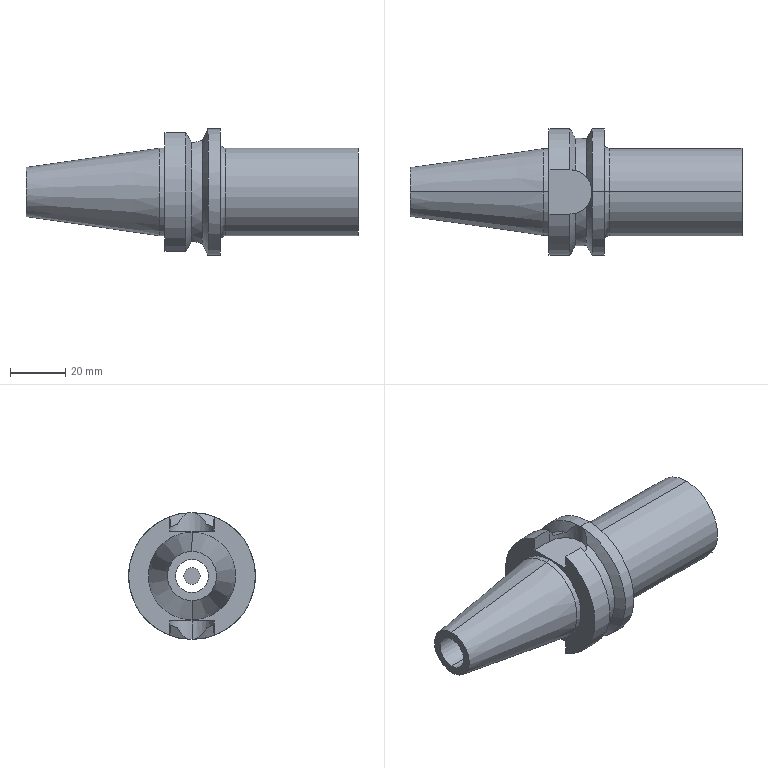Part | SolidWorks | features ICE 5, Fillet 1, MirrorPattern 1, RefAxis 1, Revolution 1 | 2 solids | 40 faces | box 120.4 x 46 x 46 mm | volume 69900 mm3 | cylinder 19 | plane 13 | cone 6 | torus 2 | commonest cylinder face diameters 46 x4 16.1 x3 6 x2 12 x2 24 x2 31.75 x2
STEP:
#1=CARTESIAN_POINT('',(90.4,0.,12.));
#2=VERTEX_POINT('',#1);
#3=CARTESIAN_POINT('',(90.4,0.,-12.));
#4=VERTEX_POINT('',#3);
#5=CARTESIAN_POINT('',(90.4,0.,0.));
#6=DIRECTION('',(1.,0.,0.));
#7=DIRECTION('',(0.,0.,-1.));
#8=AXIS2_PLACEMENT_3D('',#5,#6,#7);
#9=CIRCLE('',#8,12.);
#10=EDGE_CURVE('',#2,#4,#9,.T.);
#11=ORIENTED_EDGE('',*,*,#10,.F.);
#12=CARTESIAN_POINT('',(120.4,0.,12.));
#13=VERTEX_POINT('',#12);
#14=CARTESIAN_POINT('',(90.4,0.,12.));
#15=DIRECTION('',(1.,0.,0.));
#16=VECTOR('',#15,1000.);
#17=LINE('',#14,#16);
#18=EDGE_CURVE('',#2,#13,#17,.T.);
#19=ORIENTED_EDGE('',*,*,#18,.T.);
#20=CARTESIAN_POINT('',(120.4,0.,-12.));
#21=VERTEX_POINT('',#20);
#22=CARTESIAN_POINT('',(120.4,0.,0.));
#23=DIRECTION('',(1.,0.,0.));
#24=DIRECTION('',(0.,0.,-1.));
#25=AXIS2_PLACEMENT_3D('',#22,#23,#24);
#26=CIRCLE('',#25,12.);
#27=EDGE_CURVE('',#13,#21,#26,.T.);
#28=ORIENTED_EDGE('',*,*,#27,.T.);
#29=CARTESIAN_POINT('',(90.4,0.,-12.));
#30=DIRECTION('',(1.,0.,0.));
#31=VECTOR('',#30,1000.);
#32=LINE('',#29,#31);
#33=EDGE_CURVE('',#4,#21,#32,.T.);
#34=ORIENTED_EDGE('',*,*,#33,.F.);
#35=EDGE_LOOP('',(#11,#19,#28,#34));
#36=FACE_OUTER_BOUND('',#35,.T.);
#37=CARTESIAN_POINT('',(90.4,0.,0.));
#38=DIRECTION('',(1.,0.,0.));
#39=DIRECTION('',(0.,0.,-1.));
#40=AXIS2_PLACEMENT_3D('',#37,#38,#39);
#41=CYLINDRICAL_SURFACE('',#40,12.);
#42=ADVANCED_FACE('',(#36),#41,.F.);
#43=CARTESIAN_POINT('',(72.4,0.,15.9));
#44=VERTEX_POINT('',#43);
#45=CARTESIAN_POINT('',(72.4,0.,-15.9));
#46=VERTEX_POINT('',#45);
#47=CARTESIAN_POINT('',(72.4,0.,0.));
#48=DIRECTION('',(1.,0.,0.));
#49=DIRECTION('',(0.,0.,-1.));
#50=AXIS2_PLACEMENT_3D('',#47,#48,#49);
#51=CIRCLE('',#50,15.9);
#52=EDGE_CURVE('',#44,#46,#51,.T.);
#53=ORIENTED_EDGE('',*,*,#52,.F.);
#54=CARTESIAN_POINT('',(70.4,0.,17.9));
#55=VERTEX_POINT('',#54);
#56=CARTESIAN_POINT('',(72.4,0.,17.9));
#57=DIRECTION('',(0.,1.,0.));
#58=DIRECTION('',(0.,0.,1.));
#59=AXIS2_PLACEMENT_3D('',#56,#57,#58);
#60=CIRCLE('',#59,2.);
#61=EDGE_CURVE('',#44,#55,#60,.T.);
#62=ORIENTED_EDGE('',*,*,#61,.T.);
#63=CARTESIAN_POINT('',(70.4,0.,-17.9));
#64=VERTEX_POINT('',#63);
#65=CARTESIAN_POINT('',(70.4,0.,0.));
#66=DIRECTION('',(-1.,0.,0.));
#67=DIRECTION('',(0.,0.,-1.));
#68=AXIS2_PLACEMENT_3D('',#65,#66,#67);
#69=CIRCLE('',#68,17.9);
#70=EDGE_CURVE('',#64,#55,#69,.T.);
#71=ORIENTED_EDGE('',*,*,#70,.F.);
#72=CARTESIAN_POINT('',(72.4,0.,-17.9));
#73=DIRECTION('',(0.,-1.,0.));
#74=DIRECTION('',(0.,0.,-1.));
#75=AXIS2_PLACEMENT_3D('',#72,#73,#74);
#76=CIRCLE('',#75,2.);
#77=EDGE_CURVE('',#46,#64,#76,.T.);
#78=ORIENTED_EDGE('',*,*,#77,.F.);
#79=EDGE_LOOP('',(#53,#62,#71,#78));
#80=FACE_OUTER_BOUND('',#79,.T.);
#81=CARTESIAN_POINT('',(72.4,0.,0.));
#82=DIRECTION('',(1.,0.,0.));
#83=DIRECTION('',(0.,0.,-1.));
#84=AXIS2_PLACEMENT_3D('',#81,#82,#83);
#85=TOROIDAL_SURFACE('',#84,17.9,2.);
#86=ADVANCED_FACE('',(#80),#85,.F.);
#87=CARTESIAN_POINT('',(120.4,0.,-15.9));
#88=VERTEX_POINT('',#87);
#89=CARTESIAN_POINT('',(120.4,0.,15.9));
#90=VERTEX_POINT('',#89);
#91=CARTESIAN_POINT('',(120.4,0.,0.));
#92=DIRECTION('',(1.,0.,0.));
#93=DIRECTION('',(0.,0.,-1.));
#94=AXIS2_PLACEMENT_3D('',#91,#92,#93);
#95=CIRCLE('',#94,15.9);
#96=EDGE_CURVE('',#88,#90,#95,.T.);
#97=ORIENTED_EDGE('',*,*,#96,.F.);
#98=CARTESIAN_POINT('',(120.4,0.,-15.9));
#99=DIRECTION('',(-1.,0.,0.));
#100=VECTOR('',#99,1000.);
#101=LINE('',#98,#100);
#102=EDGE_CURVE('',#88,#46,#101,.T.);
#103=ORIENTED_EDGE('',*,*,#102,.T.);
#104=CARTESIAN_POINT('',(72.4,0.,0.));
#105=DIRECTION('',(1.,0.,0.));
#106=DIRECTION('',(0.,0.,-1.));
#107=AXIS2_PLACEMENT_3D('',#104,#105,#106);
#108=CIRCLE('',#107,15.9);
#109=EDGE_CURVE('',#46,#44,#108,.T.);
#110=ORIENTED_EDGE('',*,*,#109,.T.);
#111=CARTESIAN_POINT('',(120.4,0.,15.9));
#112=DIRECTION('',(-1.,0.,0.));
#113=VECTOR('',#112,1000.);
#114=LINE('',#111,#113);
#115=EDGE_CURVE('',#90,#44,#114,.T.);
#116=ORIENTED_EDGE('',*,*,#115,.F.);
#117=EDGE_LOOP('',(#97,#103,#110,#116));
#118=FACE_OUTER_BOUND('',#117,.T.);
#119=CARTESIAN_POINT('',(120.4,0.,0.));
#120=DIRECTION('',(-1.,0.,0.));
#121=DIRECTION('',(0.,0.,1.));
#122=AXIS2_PLACEMENT_3D('',#119,#120,#121);
#123=CYLINDRICAL_SURFACE('',#122,15.9);
#124=ADVANCED_FACE('',(#118),#123,.T.);
#125=CARTESIAN_POINT('',(66.029,0.,-22.999));
#126=VERTEX_POINT('',#125);
#127=CARTESIAN_POINT('',(66.021,0.3709,-22.997));
#128=VERTEX_POINT('',#127);
#129=CARTESIAN_POINT('',(66.029,0.,-22.999));
#130=CARTESIAN_POINT('',(66.029,0.1237,-23.));
#131=CARTESIAN_POINT('',(66.026,0.2473,-22.999));
#132=CARTESIAN_POINT('',(66.021,0.3709,-22.997));
#133=B_SPLINE_CURVE_WITH_KNOTS('',3,(#129,#130,#131,#132),.UNSPECIFIED.,.F.,.F.,(4,4),(0.5,1.),.UNSPECIFIED.);
#134=EDGE_CURVE('',#126,#128,#133,.T.);
#135=ORIENTED_EDGE('',*,*,#134,.F.);
#136=CARTESIAN_POINT('',(66.029,0.,-16.3));
#137=VERTEX_POINT('',#136);
#138=CARTESIAN_POINT('',(66.029,0.,-26.3));
#139=DIRECTION('',(0.,0.,1.));
#140=VECTOR('',#139,1000.);
#141=LINE('',#138,#140);
#142=EDGE_CURVE('',#126,#137,#141,.T.);
#143=ORIENTED_EDGE('',*,*,#142,.T.);
#144=CARTESIAN_POINT('',(57.979,8.05,-16.3));
#145=VERTEX_POINT('',#144);
#146=CARTESIAN_POINT('',(57.979,0.,-16.3));
#147=DIRECTION('',(0.,0.,1.));
#148=DIRECTION('',(1.,0.,0.));
#149=AXIS2_PLACEMENT_3D('',#146,#147,#148);
#150=CIRCLE('',#149,8.05);
#151=EDGE_CURVE('',#137,#145,#150,.T.);
#152=ORIENTED_EDGE('',*,*,#151,.T.);
#153=CARTESIAN_POINT('',(57.979,8.05,-21.545));
#154=VERTEX_POINT('',#153);
#155=CARTESIAN_POINT('',(57.979,8.05,-26.3));
#156=DIRECTION('',(0.,0.,1.));
#157=VECTOR('',#156,1000.);
#158=LINE('',#155,#157);
#159=EDGE_CURVE('',#154,#145,#158,.T.);
#160=ORIENTED_EDGE('',*,*,#159,.F.);
#161=CARTESIAN_POINT('',(60.,7.792,-17.875));
#162=VERTEX_POINT('',#161);
#163=CARTESIAN_POINT('',(57.979,8.05,-21.545));
#164=CARTESIAN_POINT('',(58.646,8.05,-20.312));
#165=CARTESIAN_POINT('',(59.318,7.969,-19.087));
#166=CARTESIAN_POINT('',(60.,7.792,-17.875));
#167=B_SPLINE_CURVE_WITH_KNOTS('',3,(#163,#164,#165,#166),.UNSPECIFIED.,.F.,.F.,(4,4),(0.0004247,0.004622),.UNSPECIFIED.);
#168=EDGE_CURVE('',#154,#162,#167,.T.);
#169=ORIENTED_EDGE('',*,*,#168,.T.);
#170=CARTESIAN_POINT('',(64.,5.344,-18.754));
#171=VERTEX_POINT('',#170);
#172=CARTESIAN_POINT('',(60.,7.792,-17.875));
#173=CARTESIAN_POINT('',(60.783,7.589,-17.964));
#174=CARTESIAN_POINT('',(61.51,7.278,-18.096));
#175=CARTESIAN_POINT('',(62.524,6.656,-18.33));
#176=CARTESIAN_POINT('',(62.848,6.423,-18.414));
#177=CARTESIAN_POINT('',(63.453,5.916,-18.583));
#178=CARTESIAN_POINT('',(63.736,5.641,-18.669));
#179=CARTESIAN_POINT('',(64.,5.344,-18.754));
#180=B_SPLINE_CURVE_WITH_KNOTS('',3,(#172,#173,#174,#175,#176,#177,#178,#179),.UNSPECIFIED.,.F.,.F.,(4,2,2,4),(0.,0.002405,0.003607,0.004809),.UNSPECIFIED.);
#181=EDGE_CURVE('',#162,#171,#180,.T.);
#182=ORIENTED_EDGE('',*,*,#181,.T.);
#183=CARTESIAN_POINT('',(64.,5.344,-18.754));
#184=CARTESIAN_POINT('',(64.227,5.088,-19.234));
#185=CARTESIAN_POINT('',(64.448,4.807,-19.703));
#186=CARTESIAN_POINT('',(64.876,4.169,-20.605));
#187=CARTESIAN_POINT('',(65.084,3.81,-21.041));
#188=CARTESIAN_POINT('',(65.461,3.003,-21.83));
#189=CARTESIAN_POINT('',(65.633,2.548,-22.189));
#190=CARTESIAN_POINT('',(65.832,1.79,-22.604));
#191=CARTESIAN_POINT('',(65.889,1.522,-22.723));
#192=CARTESIAN_POINT('',(65.977,0.957,-22.907));
#193=CARTESIAN_POINT('',(66.007,0.6678,-22.968));
#194=CARTESIAN_POINT('',(66.021,0.3709,-22.997));
#195=B_SPLINE_CURVE_WITH_KNOTS('',3,(#183,#184,#185,#186,#187,#188,#189,#190,#191,#192,#193,#194),.UNSPECIFIED.,.F.,.F.,(4,2,2,2,2,4),(0.002168,0.003936,0.005704,0.007473,0.008357,0.009241),.UNSPECIFIED.);
#196=EDGE_CURVE('',#171,#128,#195,.T.);
#197=ORIENTED_EDGE('',*,*,#196,.T.);
#198=EDGE_LOOP('',(#135,#143,#152,#160,#169,#182,#197));
#199=FACE_OUTER_BOUND('',#198,.T.);
#200=CARTESIAN_POINT('',(57.979,0.,-26.3));
#201=DIRECTION('',(0.,0.,1.));
#202=DIRECTION('',(1.,0.,0.));
#203=AXIS2_PLACEMENT_3D('',#200,#201,#202);
#204=CYLINDRICAL_SURFACE('',#203,8.05);
#205=ADVANCED_FACE('',(#199),#204,.F.);
#206=CARTESIAN_POINT('',(48.4,0.,-15.875));
#207=VERTEX_POINT('',#206);
#208=CARTESIAN_POINT('',(48.4,0.,15.875));
#209=VERTEX_POINT('',#208);
#210=CARTESIAN_POINT('',(48.4,0.,0.));
#211=DIRECTION('',(1.,0.,0.));
#212=DIRECTION('',(0.,0.,-1.));
#213=AXIS2_PLACEMENT_3D('',#210,#211,#212);
#214=CIRCLE('',#213,15.875);
#215=EDGE_CURVE('',#207,#209,#214,.T.);
#216=ORIENTED_EDGE('',*,*,#215,.T.);
#217=CARTESIAN_POINT('',(50.4,0.,15.875));
#218=VERTEX_POINT('',#217);
#219=CARTESIAN_POINT('',(70.4,0.,15.875));
#220=DIRECTION('',(1.,0.,0.));
#221=VECTOR('',#220,1000.);
#222=LINE('',#219,#221);
#223=EDGE_CURVE('',#209,#218,#222,.T.);
#224=ORIENTED_EDGE('',*,*,#223,.T.);
#225=CARTESIAN_POINT('',(50.4,0.,-15.875));
#226=VERTEX_POINT('',#225);
#227=CARTESIAN_POINT('',(50.4,0.,0.));
#228=DIRECTION('',(1.,0.,0.));
#229=DIRECTION('',(0.,0.,-1.));
#230=AXIS2_PLACEMENT_3D('',#227,#228,#229);
#231=CIRCLE('',#230,15.875);
#232=EDGE_CURVE('',#226,#218,#231,.T.);
#233=ORIENTED_EDGE('',*,*,#232,.F.);
#234=CARTESIAN_POINT('',(70.4,0.,-15.875));
#235=DIRECTION('',(1.,0.,0.));
#236=VECTOR('',#235,1000.);
#237=LINE('',#234,#236);
#238=EDGE_CURVE('',#207,#226,#237,.T.);
#239=ORIENTED_EDGE('',*,*,#238,.F.);
#240=EDGE_LOOP('',(#216,#224,#233,#239));
#241=FACE_OUTER_BOUND('',#240,.T.);
#242=CARTESIAN_POINT('',(70.4,0.,0.));
#243=DIRECTION('',(1.,0.,0.));
#244=DIRECTION('',(0.,0.,-1.));
#245=AXIS2_PLACEMENT_3D('',#242,#243,#244);
#246=CYLINDRICAL_SURFACE('',#245,15.875);
#247=ADVANCED_FACE('',(#241),#246,.T.);
#248=CARTESIAN_POINT('',(0.,0.,-8.922));
#249=VERTEX_POINT('',#248);
#250=CARTESIAN_POINT('',(0.,0.,8.922));
#251=VERTEX_POINT('',#250);
#252=CARTESIAN_POINT('',(0.,0.,0.));
#253=DIRECTION('',(1.,0.,0.));
#254=DIRECTION('',(0.,0.,-1.));
#255=AXIS2_PLACEMENT_3D('',#252,#253,#254);
#256=CIRCLE('',#255,8.922);
#257=EDGE_CURVE('',#249,#251,#256,.T.);
#258=ORIENTED_EDGE('',*,*,#257,.T.);
#259=CARTESIAN_POINT('',(48.4,0.,15.875));
#260=DIRECTION('',(0.9898,0.,0.1422));
#261=VECTOR('',#260,1000.);
#262=LINE('',#259,#261);
#263=EDGE_CURVE('',#251,#209,#262,.T.);
#264=ORIENTED_EDGE('',*,*,#263,.T.);
#265=ORIENTED_EDGE('',*,*,#215,.F.);
#266=CARTESIAN_POINT('',(48.4,0.,-15.875));
#267=DIRECTION('',(0.9898,0.,-0.1422));
#268=VECTOR('',#267,1000.);
#269=LINE('',#266,#268);
#270=EDGE_CURVE('',#249,#207,#269,.T.);
#271=ORIENTED_EDGE('',*,*,#270,.F.);
#272=EDGE_LOOP('',(#258,#264,#265,#271));
#273=FACE_OUTER_BOUND('',#272,.T.);
#274=CARTESIAN_POINT('',(48.4,0.,0.));
#275=DIRECTION('',(1.,0.,0.));
#276=DIRECTION('',(0.,0.,-1.));
#277=AXIS2_PLACEMENT_3D('',#274,#275,#276);
#278=CONICAL_SURFACE('',#277,15.875,0.1427);
#279=ADVANCED_FACE('',(#273),#278,.T.);
#280=CARTESIAN_POINT('',(66.021,0.3709,22.997));
#281=VERTEX_POINT('',#280);
#282=CARTESIAN_POINT('',(66.029,0.,22.999));
#283=VERTEX_POINT('',#282);
#284=CARTESIAN_POINT('',(66.021,0.3709,22.997));
#285=CARTESIAN_POINT('',(66.026,0.2473,22.999));
#286=CARTESIAN_POINT('',(66.029,0.1236,23.));
#287=CARTESIAN_POINT('',(66.029,0.,22.999));
#288=B_SPLINE_CURVE_WITH_KNOTS('',3,(#284,#285,#286,#287),.UNSPECIFIED.,.F.,.F.,(4,4),(0.,0.5),.UNSPECIFIED.);
#289=EDGE_CURVE('',#281,#283,#288,.T.);
#290=ORIENTED_EDGE('',*,*,#289,.T.);
#291=CARTESIAN_POINT('',(70.4,0.,23.));
#292=VERTEX_POINT('',#291);
#293=CARTESIAN_POINT('',(70.4,0.,23.));
#294=DIRECTION('',(1.,0.,0.));
#295=VECTOR('',#294,1000.);
#296=LINE('',#293,#295);
#297=EDGE_CURVE('',#283,#292,#296,.T.);
#298=ORIENTED_EDGE('',*,*,#297,.T.);
#299=CARTESIAN_POINT('',(70.4,0.,-23.));
#300=VERTEX_POINT('',#299);
#301=CARTESIAN_POINT('',(70.4,0.,0.));
#302=DIRECTION('',(1.,0.,0.));
#303=DIRECTION('',(0.,0.,-1.));
#304=AXIS2_PLACEMENT_3D('',#301,#302,#303);
#305=CIRCLE('',#304,23.);
#306=EDGE_CURVE('',#300,#292,#305,.T.);
#307=ORIENTED_EDGE('',*,*,#306,.F.);
#308=CARTESIAN_POINT('',(70.4,0.,-23.));
#309=DIRECTION('',(1.,0.,0.));
#310=VECTOR('',#309,1000.);
#311=LINE('',#308,#310);
#312=EDGE_CURVE('',#126,#300,#311,.T.);
#313=ORIENTED_EDGE('',*,*,#312,.F.);
#314=ORIENTED_EDGE('',*,*,#134,.T.);
#315=CARTESIAN_POINT('',(66.021,0.,0.));
#316=DIRECTION('',(1.,0.,0.));
#317=DIRECTION('',(0.,0.,-1.));
#318=AXIS2_PLACEMENT_3D('',#315,#316,#317);
#319=CIRCLE('',#318,23.);
#320=EDGE_CURVE('',#128,#281,#319,.T.);
#321=ORIENTED_EDGE('',*,*,#320,.T.);
#322=EDGE_LOOP('',(#290,#298,#307,#313,#314,#321));
#323=FACE_OUTER_BOUND('',#322,.T.);
#324=CARTESIAN_POINT('',(70.4,0.,0.));
#325=DIRECTION('',(1.,0.,0.));
#326=DIRECTION('',(0.,0.,-1.));
#327=AXIS2_PLACEMENT_3D('',#324,#325,#326);
#328=CYLINDRICAL_SURFACE('',#327,23.);
#329=ADVANCED_FACE('',(#323),#328,.T.);
#330=CARTESIAN_POINT('',(90.4,0.,-6.));
#331=VERTEX_POINT('',#330);
#332=CARTESIAN_POINT('',(90.4,0.,6.));
#333=VERTEX_POINT('',#332);
#334=CARTESIAN_POINT('',(90.4,0.,0.));
#335=DIRECTION('',(-1.,0.,0.));
#336=DIRECTION('',(0.,0.,-1.));
#337=AXIS2_PLACEMENT_3D('',#334,#335,#336);
#338=CIRCLE('',#337,6.);
#339=EDGE_CURVE('',#331,#333,#338,.T.);
#340=ORIENTED_EDGE('',*,*,#339,.F.);
#341=CARTESIAN_POINT('',(0.,0.,-6.));
#342=VERTEX_POINT('',#341);
#343=CARTESIAN_POINT('',(120.4,0.,-6.));
#344=DIRECTION('',(-1.,0.,0.));
#345=VECTOR('',#344,1000.);
#346=LINE('',#343,#345);
#347=EDGE_CURVE('',#331,#342,#346,.T.);
#348=ORIENTED_EDGE('',*,*,#347,.T.);
#349=CARTESIAN_POINT('',(0.,0.,6.));
#350=VERTEX_POINT('',#349);
#351=CARTESIAN_POINT('',(0.,0.,0.));
#352=DIRECTION('',(-1.,0.,0.));
#353=DIRECTION('',(0.,0.,1.));
#354=AXIS2_PLACEMENT_3D('',#351,#352,#353);
#355=CIRCLE('',#354,6.);
#356=EDGE_CURVE('',#342,#350,#355,.T.);
#357=ORIENTED_EDGE('',*,*,#356,.T.);
#358=CARTESIAN_POINT('',(120.4,0.,6.));
#359=DIRECTION('',(-1.,0.,0.));
#360=VECTOR('',#359,1000.);
#361=LINE('',#358,#360);
#362=EDGE_CURVE('',#333,#350,#361,.T.);
#363=ORIENTED_EDGE('',*,*,#362,.F.);
#364=EDGE_LOOP('',(#340,#348,#357,#363));
#365=FACE_OUTER_BOUND('',#364,.T.);
#366=CARTESIAN_POINT('',(120.4,0.,0.));
#367=DIRECTION('',(-1.,0.,0.));
#368=DIRECTION('',(0.,0.,1.));
#369=AXIS2_PLACEMENT_3D('',#366,#367,#368);
#370=CYLINDRICAL_SURFACE('',#369,6.);
#371=ADVANCED_FACE('',(#365),#370,.F.);
#372=ORIENTED_EDGE('',*,*,#347,.F.);
#373=CARTESIAN_POINT('',(90.4,0.,0.));
#374=DIRECTION('',(-1.,0.,0.));
#375=DIRECTION('',(0.,0.,-1.));
#376=AXIS2_PLACEMENT_3D('',#373,#374,#375);
#377=CIRCLE('',#376,6.);
#378=EDGE_CURVE('',#333,#331,#377,.T.);
#379=ORIENTED_EDGE('',*,*,#378,.F.);
#380=ORIENTED_EDGE('',*,*,#362,.T.);
#381=CARTESIAN_POINT('',(0.,0.,0.));
#382=DIRECTION('',(-1.,0.,0.));
#383=DIRECTION('',(0.,0.,1.));
#384=AXIS2_PLACEMENT_3D('',#381,#382,#383);
#385=CIRCLE('',#384,6.);
#386=EDGE_CURVE('',#350,#342,#385,.T.);
#387=ORIENTED_EDGE('',*,*,#386,.T.);
#388=EDGE_LOOP('',(#372,#379,#380,#387));
#389=FACE_OUTER_BOUND('',#388,.T.);
#390=CARTESIAN_POINT('',(120.4,0.,0.));
#391=DIRECTION('',(-1.,0.,0.));
#392=DIRECTION('',(0.,0.,1.));
#393=AXIS2_PLACEMENT_3D('',#390,#391,#392);
#394=CYLINDRICAL_SURFACE('',#393,6.);
#395=ADVANCED_FACE('',(#389),#394,.F.);
#396=CARTESIAN_POINT('',(57.979,-8.05,-21.545));
#397=VERTEX_POINT('',#396);
#398=CARTESIAN_POINT('',(50.4,-8.05,-21.545));
#399=VERTEX_POINT('',#398);
#400=CARTESIAN_POINT('',(70.4,-8.05,-21.545));
#401=DIRECTION('',(-1.,0.,0.));
#402=VECTOR('',#401,1000.);
#403=LINE('',#400,#402);
#404=EDGE_CURVE('',#397,#399,#403,.T.);
#405=ORIENTED_EDGE('',*,*,#404,.F.);
#406=CARTESIAN_POINT('',(57.979,-8.05,21.545));
#407=VERTEX_POINT('',#406);
#408=CARTESIAN_POINT('',(57.979,0.,0.));
#409=DIRECTION('',(1.,0.,0.));
#410=DIRECTION('',(0.,0.,-1.));
#411=AXIS2_PLACEMENT_3D('',#408,#409,#410);
#412=CIRCLE('',#411,23.);
#413=EDGE_CURVE('',#407,#397,#412,.T.);
#414=ORIENTED_EDGE('',*,*,#413,.F.);
#415=CARTESIAN_POINT('',(50.4,-8.05,21.545));
#416=VERTEX_POINT('',#415);
#417=CARTESIAN_POINT('',(70.4,-8.05,21.545));
#418=DIRECTION('',(-1.,0.,0.));
#419=VECTOR('',#418,1000.);
#420=LINE('',#417,#419);
#421=EDGE_CURVE('',#407,#416,#420,.T.);
#422=ORIENTED_EDGE('',*,*,#421,.T.);
#423=CARTESIAN_POINT('',(50.4,0.,0.));
#424=DIRECTION('',(1.,0.,0.));
#425=DIRECTION('',(0.,0.,-1.));
#426=AXIS2_PLACEMENT_3D('',#423,#424,#425);
#427=CIRCLE('',#426,23.);
#428=EDGE_CURVE('',#416,#399,#427,.T.);
#429=ORIENTED_EDGE('',*,*,#428,.T.);
#430=EDGE_LOOP('',(#405,#414,#422,#429));
#431=FACE_OUTER_BOUND('',#430,.T.);
#432=CARTESIAN_POINT('',(70.4,0.,0.));
#433=DIRECTION('',(1.,0.,0.));
#434=DIRECTION('',(0.,0.,-1.));
#435=AXIS2_PLACEMENT_3D('',#432,#433,#434);
#436=CYLINDRICAL_SURFACE('',#435,23.);
#437=ADVANCED_FACE('',(#431),#436,.T.);
#438=CARTESIAN_POINT('',(60.,-7.792,-17.875));
#439=VERTEX_POINT('',#438);
#440=CARTESIAN_POINT('',(60.,-7.792,-17.875));
#441=CARTESIAN_POINT('',(59.318,-7.969,-19.087));
#442=CARTESIAN_POINT('',(58.646,-8.05,-20.312));
#443=CARTESIAN_POINT('',(57.979,-8.05,-21.545));
#444=B_SPLINE_CURVE_WITH_KNOTS('',3,(#440,#441,#442,#443),.UNSPECIFIED.,.F.,.F.,(4,4),(0.0004141,0.004611),.UNSPECIFIED.);
#445=EDGE_CURVE('',#439,#397,#444,.T.);
#446=ORIENTED_EDGE('',*,*,#445,.F.);
#447=CARTESIAN_POINT('',(60.,-7.792,17.875));
#448=VERTEX_POINT('',#447);
#449=CARTESIAN_POINT('',(60.,0.,0.));
#450=DIRECTION('',(1.,0.,0.));
#451=DIRECTION('',(0.,0.,-1.));
#452=AXIS2_PLACEMENT_3D('',#449,#450,#451);
#453=CIRCLE('',#452,19.5);
#454=EDGE_CURVE('',#448,#439,#453,.T.);
#455=ORIENTED_EDGE('',*,*,#454,.F.);
#456=CARTESIAN_POINT('',(60.,-7.792,17.875));
#457=CARTESIAN_POINT('',(59.318,-7.969,19.087));
#458=CARTESIAN_POINT('',(58.646,-8.05,20.312));
#459=CARTESIAN_POINT('',(57.979,-8.05,21.545));
#460=B_SPLINE_CURVE_WITH_KNOTS('',3,(#456,#457,#458,#459),.UNSPECIFIED.,.F.,.F.,(4,4),(0.0004141,0.004611),.UNSPECIFIED.);
#461=EDGE_CURVE('',#448,#407,#460,.T.);
#462=ORIENTED_EDGE('',*,*,#461,.T.);
#463=ORIENTED_EDGE('',*,*,#413,.T.);
#464=EDGE_LOOP('',(#446,#455,#462,#463));
#465=FACE_OUTER_BOUND('',#464,.T.);
#466=CARTESIAN_POINT('',(60.,0.,0.));
#467=DIRECTION('',(-1.,0.,0.));
#468=DIRECTION('',(0.,0.,1.));
#469=AXIS2_PLACEMENT_3D('',#466,#467,#468);
#470=CONICAL_SURFACE('',#469,19.5,1.047);
#471=ADVANCED_FACE('',(#465),#470,.T.);
#472=ORIENTED_EDGE('',*,*,#181,.F.);
#473=CARTESIAN_POINT('',(60.,7.792,17.875));
#474=VERTEX_POINT('',#473);
#475=CARTESIAN_POINT('',(60.,0.,0.));
#476=DIRECTION('',(1.,0.,0.));
#477=DIRECTION('',(0.,0.,-1.));
#478=AXIS2_PLACEMENT_3D('',#475,#476,#477);
#479=CIRCLE('',#478,19.5);
#480=EDGE_CURVE('',#162,#474,#479,.T.);
#481=ORIENTED_EDGE('',*,*,#480,.T.);
#482=CARTESIAN_POINT('',(64.,5.344,18.754));
#483=VERTEX_POINT('',#482);
#484=CARTESIAN_POINT('',(60.,7.792,17.875));
#485=CARTESIAN_POINT('',(60.783,7.589,17.964));
#486=CARTESIAN_POINT('',(61.51,7.278,18.096));
#487=CARTESIAN_POINT('',(62.524,6.656,18.33));
#488=CARTESIAN_POINT('',(62.848,6.423,18.414));
#489=CARTESIAN_POINT('',(63.453,5.916,18.583));
#490=CARTESIAN_POINT('',(63.736,5.641,18.669));
#491=CARTESIAN_POINT('',(64.,5.344,18.754));
#492=B_SPLINE_CURVE_WITH_KNOTS('',3,(#484,#485,#486,#487,#488,#489,#490,#491),.UNSPECIFIED.,.F.,.F.,(4,2,2,4),(0.,0.002405,0.003607,0.004809),.UNSPECIFIED.);
#493=EDGE_CURVE('',#474,#483,#492,.T.);
#494=ORIENTED_EDGE('',*,*,#493,.T.);
#495=CARTESIAN_POINT('',(64.,0.,0.));
#496=DIRECTION('',(1.,0.,0.));
#497=DIRECTION('',(0.,0.,-1.));
#498=AXIS2_PLACEMENT_3D('',#495,#496,#497);
#499=CIRCLE('',#498,19.5);
#500=EDGE_CURVE('',#171,#483,#499,.T.);
#501=ORIENTED_EDGE('',*,*,#500,.F.);
#502=EDGE_LOOP('',(#472,#481,#494,#501));
#503=FACE_OUTER_BOUND('',#502,.T.);
#504=CARTESIAN_POINT('',(70.4,0.,0.));
#505=DIRECTION('',(1.,0.,0.));
#506=DIRECTION('',(0.,0.,-1.));
#507=AXIS2_PLACEMENT_3D('',#504,#505,#506);
#508=CYLINDRICAL_SURFACE('',#507,19.5);
#509=ADVANCED_FACE('',(#503),#508,.T.);
#510=ORIENTED_EDGE('',*,*,#196,.F.);
#511=ORIENTED_EDGE('',*,*,#500,.T.);
#512=CARTESIAN_POINT('',(64.,5.344,18.754));
#513=CARTESIAN_POINT('',(64.228,5.087,19.237));
#514=CARTESIAN_POINT('',(64.45,4.804,19.706));
#515=CARTESIAN_POINT('',(64.876,4.17,20.603));
#516=CARTESIAN_POINT('',(65.08,3.818,21.032));
#517=CARTESIAN_POINT('',(65.365,3.209,21.629));
#518=CARTESIAN_POINT('',(65.455,2.995,21.817));
#519=CARTESIAN_POINT('',(65.622,2.541,22.165));
#520=CARTESIAN_POINT('',(65.699,2.298,22.326));
#521=CARTESIAN_POINT('',(65.833,1.788,22.605));
#522=CARTESIAN_POINT('',(65.889,1.522,22.723));
#523=CARTESIAN_POINT('',(65.976,0.9634,22.905));
#524=CARTESIAN_POINT('',(66.007,0.6669,22.969));
#525=CARTESIAN_POINT('',(66.021,0.3709,22.997));
#526=B_SPLINE_CURVE_WITH_KNOTS('',3,(#512,#513,#514,#515,#516,#517,#518,#519,#520,#521,#522,#523,#524,#525),.UNSPECIFIED.,.F.,.F.,(4,2,2,2,2,2,4),(0.0005191,0.002287,0.004055,0.004939,0.005823,0.006707,0.007591),.UNSPECIFIED.);
#527=EDGE_CURVE('',#483,#281,#526,.T.);
#528=ORIENTED_EDGE('',*,*,#527,.T.);
#529=ORIENTED_EDGE('',*,*,#320,.F.);
#530=EDGE_LOOP('',(#510,#511,#528,#529));
#531=FACE_OUTER_BOUND('',#530,.T.);
#532=CARTESIAN_POINT('',(66.021,0.,0.));
#533=DIRECTION('',(1.,0.,0.));
#534=DIRECTION('',(0.,0.,-1.));
#535=AXIS2_PLACEMENT_3D('',#532,#533,#534);
#536=CONICAL_SURFACE('',#535,23.,1.047);
#537=ADVANCED_FACE('',(#531),#536,.T.);
#538=CARTESIAN_POINT('',(50.4,-8.05,-16.3));
#539=VERTEX_POINT('',#538);
#540=CARTESIAN_POINT('',(50.4,-8.05,-26.3));
#541=DIRECTION('',(0.,0.,1.));
#542=VECTOR('',#541,1000.);
#543=LINE('',#540,#542);
#544=EDGE_CURVE('',#399,#539,#543,.T.);
#545=ORIENTED_EDGE('',*,*,#544,.F.);
#546=ORIENTED_EDGE('',*,*,#428,.F.);
#547=CARTESIAN_POINT('',(50.4,-8.05,16.3));
#548=VERTEX_POINT('',#547);
#549=CARTESIAN_POINT('',(50.4,-8.05,26.3));
#550=DIRECTION('',(0.,0.,-1.));
#551=VECTOR('',#550,1000.);
#552=LINE('',#549,#551);
#553=EDGE_CURVE('',#416,#548,#552,.T.);
#554=ORIENTED_EDGE('',*,*,#553,.T.);
#555=CARTESIAN_POINT('',(50.4,8.05,16.3));
#556=VERTEX_POINT('',#555);
#557=CARTESIAN_POINT('',(50.4,8.05,16.3));
#558=DIRECTION('',(0.,-1.,0.));
#559=VECTOR('',#558,1000.);
#560=LINE('',#557,#559);
#561=EDGE_CURVE('',#556,#548,#560,.T.);
#562=ORIENTED_EDGE('',*,*,#561,.F.);
#563=CARTESIAN_POINT('',(50.4,8.05,21.545));
#564=VERTEX_POINT('',#563);
#565=CARTESIAN_POINT('',(50.4,8.05,26.3));
#566=DIRECTION('',(0.,0.,-1.));
#567=VECTOR('',#566,1000.);
#568=LINE('',#565,#567);
#569=EDGE_CURVE('',#564,#556,#568,.T.);
#570=ORIENTED_EDGE('',*,*,#569,.F.);
#571=CARTESIAN_POINT('',(50.4,8.05,-21.545));
#572=VERTEX_POINT('',#571);
#573=CARTESIAN_POINT('',(50.4,0.,0.));
#574=DIRECTION('',(1.,0.,0.));
#575=DIRECTION('',(0.,0.,-1.));
#576=AXIS2_PLACEMENT_3D('',#573,#574,#575);
#577=CIRCLE('',#576,23.);
#578=EDGE_CURVE('',#572,#564,#577,.T.);
#579=ORIENTED_EDGE('',*,*,#578,.F.);
#580=CARTESIAN_POINT('',(50.4,8.05,-16.3));
#581=VERTEX_POINT('',#580);
#582=CARTESIAN_POINT('',(50.4,8.05,-26.3));
#583=DIRECTION('',(0.,0.,1.));
#584=VECTOR('',#583,1000.);
#585=LINE('',#582,#584);
#586=EDGE_CURVE('',#572,#581,#585,.T.);
#587=ORIENTED_EDGE('',*,*,#586,.T.);
#588=CARTESIAN_POINT('',(50.4,8.05,-16.3));
#589=DIRECTION('',(0.,-1.,0.));
#590=VECTOR('',#589,1000.);
#591=LINE('',#588,#590);
#592=EDGE_CURVE('',#581,#539,#591,.T.);
#593=ORIENTED_EDGE('',*,*,#592,.T.);
#594=EDGE_LOOP('',(#545,#546,#554,#562,#570,#579,#587,#593));
#595=FACE_OUTER_BOUND('',#594,.T.);
#596=ORIENTED_EDGE('',*,*,#232,.T.);
#597=CARTESIAN_POINT('',(50.4,0.,0.));
#598=DIRECTION('',(1.,0.,0.));
#599=DIRECTION('',(0.,0.,-1.));
#600=AXIS2_PLACEMENT_3D('',#597,#598,#599);
#601=CIRCLE('',#600,15.875);
#602=EDGE_CURVE('',#218,#226,#601,.T.);
#603=ORIENTED_EDGE('',*,*,#602,.T.);
#604=EDGE_LOOP('',(#596,#603));
#605=FACE_BOUND('',#604,.T.);
#606=CARTESIAN_POINT('',(50.4,15.875,0.));
#607=DIRECTION('',(-1.,0.,0.));
#608=DIRECTION('',(0.,0.,1.));
#609=AXIS2_PLACEMENT_3D('',#606,#607,#608);
#610=PLANE('',#609);
#611=ADVANCED_FACE('',(#595,#605),#610,.T.);
#612=CARTESIAN_POINT('',(70.4,8.05,-21.545));
#613=DIRECTION('',(1.,0.,0.));
#614=VECTOR('',#613,1000.);
#615=LINE('',#612,#614);
#616=EDGE_CURVE('',#572,#154,#615,.T.);
#617=ORIENTED_EDGE('',*,*,#616,.F.);
#618=ORIENTED_EDGE('',*,*,#578,.T.);
#619=CARTESIAN_POINT('',(57.979,8.05,21.545));
#620=VERTEX_POINT('',#619);
#621=CARTESIAN_POINT('',(70.4,8.05,21.545));
#622=DIRECTION('',(1.,0.,0.));
#623=VECTOR('',#622,1000.);
#624=LINE('',#621,#623);
#625=EDGE_CURVE('',#564,#620,#624,.T.);
#626=ORIENTED_EDGE('',*,*,#625,.T.);
#627=CARTESIAN_POINT('',(57.979,0.,0.));
#628=DIRECTION('',(1.,0.,0.));
#629=DIRECTION('',(0.,0.,-1.));
#630=AXIS2_PLACEMENT_3D('',#627,#628,#629);
#631=CIRCLE('',#630,23.);
#632=EDGE_CURVE('',#154,#620,#631,.T.);
#633=ORIENTED_EDGE('',*,*,#632,.F.);
#634=EDGE_LOOP('',(#617,#618,#626,#633));
#635=FACE_OUTER_BOUND('',#634,.T.);
#636=CARTESIAN_POINT('',(70.4,0.,0.));
#637=DIRECTION('',(1.,0.,0.));
#638=DIRECTION('',(0.,0.,-1.));
#639=AXIS2_PLACEMENT_3D('',#636,#637,#638);
#640=CYLINDRICAL_SURFACE('',#639,23.);
#641=ADVANCED_FACE('',(#635),#640,.T.);
#642=ORIENTED_EDGE('',*,*,#168,.F.);
#643=ORIENTED_EDGE('',*,*,#632,.T.);
#644=CARTESIAN_POINT('',(57.979,8.05,21.545));
#645=CARTESIAN_POINT('',(58.646,8.05,20.312));
#646=CARTESIAN_POINT('',(59.318,7.969,19.087));
#647=CARTESIAN_POINT('',(60.,7.792,17.875));
#648=B_SPLINE_CURVE_WITH_KNOTS('',3,(#644,#645,#646,#647),.UNSPECIFIED.,.F.,.F.,(4,4),(0.0004247,0.004622),.UNSPECIFIED.);
#649=EDGE_CURVE('',#620,#474,#648,.T.);
#650=ORIENTED_EDGE('',*,*,#649,.T.);
#651=ORIENTED_EDGE('',*,*,#480,.F.);
#652=EDGE_LOOP('',(#642,#643,#650,#651));
#653=FACE_OUTER_BOUND('',#652,.T.);
#654=CARTESIAN_POINT('',(60.,0.,0.));
#655=DIRECTION('',(-1.,0.,0.));
#656=DIRECTION('',(0.,0.,1.));
#657=AXIS2_PLACEMENT_3D('',#654,#655,#656);
#658=CONICAL_SURFACE('',#657,19.5,1.047);
#659=ADVANCED_FACE('',(#653),#658,.T.);
#660=CARTESIAN_POINT('',(64.,-5.344,-18.754));
#661=VERTEX_POINT('',#660);
#662=CARTESIAN_POINT('',(64.,-5.344,-18.754));
#663=CARTESIAN_POINT('',(63.472,-5.938,-18.584));
#664=CARTESIAN_POINT('',(62.872,-6.441,-18.411));
#665=CARTESIAN_POINT('',(61.859,-7.064,-18.177));
#666=CARTESIAN_POINT('',(61.502,-7.249,-18.103));
#667=CARTESIAN_POINT('',(60.77,-7.561,-17.975));
#668=CARTESIAN_POINT('',(60.391,-7.691,-17.92));
#669=CARTESIAN_POINT('',(60.,-7.792,-17.875));
#670=B_SPLINE_CURVE_WITH_KNOTS('',3,(#662,#663,#664,#665,#666,#667,#668,#669),.UNSPECIFIED.,.F.,.F.,(4,2,2,4),(0.,0.002406,0.003609,0.004812),.UNSPECIFIED.);
#671=EDGE_CURVE('',#661,#439,#670,.T.);
#672=ORIENTED_EDGE('',*,*,#671,.F.);
#673=CARTESIAN_POINT('',(64.,-5.344,18.754));
#674=VERTEX_POINT('',#673);
#675=CARTESIAN_POINT('',(64.,0.,0.));
#676=DIRECTION('',(1.,0.,0.));
#677=DIRECTION('',(0.,0.,-1.));
#678=AXIS2_PLACEMENT_3D('',#675,#676,#677);
#679=CIRCLE('',#678,19.5);
#680=EDGE_CURVE('',#674,#661,#679,.T.);
#681=ORIENTED_EDGE('',*,*,#680,.F.);
#682=CARTESIAN_POINT('',(64.,-5.344,18.754));
#683=CARTESIAN_POINT('',(63.472,-5.938,18.584));
#684=CARTESIAN_POINT('',(62.872,-6.441,18.411));
#685=CARTESIAN_POINT('',(61.859,-7.064,18.177));
#686=CARTESIAN_POINT('',(61.502,-7.249,18.103));
#687=CARTESIAN_POINT('',(60.77,-7.561,17.975));
#688=CARTESIAN_POINT('',(60.391,-7.691,17.92));
#689=CARTESIAN_POINT('',(60.,-7.792,17.875));
#690=B_SPLINE_CURVE_WITH_KNOTS('',3,(#682,#683,#684,#685,#686,#687,#688,#689),.UNSPECIFIED.,.F.,.F.,(4,2,2,4),(0.,0.002406,0.003609,0.004812),.UNSPECIFIED.);
#691=EDGE_CURVE('',#674,#448,#690,.T.);
#692=ORIENTED_EDGE('',*,*,#691,.T.);
#693=ORIENTED_EDGE('',*,*,#454,.T.);
#694=EDGE_LOOP('',(#672,#681,#692,#693));
#695=FACE_OUTER_BOUND('',#694,.T.);
#696=CARTESIAN_POINT('',(70.4,0.,0.));
#697=DIRECTION('',(1.,0.,0.));
#698=DIRECTION('',(0.,0.,-1.));
#699=AXIS2_PLACEMENT_3D('',#696,#697,#698);
#700=CYLINDRICAL_SURFACE('',#699,19.5);
#701=ADVANCED_FACE('',(#695),#700,.T.);
#702=CARTESIAN_POINT('',(66.021,-0.3709,-22.997));
#703=VERTEX_POINT('',#702);
#704=CARTESIAN_POINT('',(66.021,-0.3709,-22.997));
#705=CARTESIAN_POINT('',(66.014,-0.5187,-22.983));
#706=CARTESIAN_POINT('',(66.003,-0.6652,-22.96));
#707=CARTESIAN_POINT('',(65.974,-0.9558,-22.899));
#708=CARTESIAN_POINT('',(65.955,-1.101,-22.86));
#709=CARTESIAN_POINT('',(65.889,-1.523,-22.723));
#710=CARTESIAN_POINT('',(65.832,-1.79,-22.604));
#711=CARTESIAN_POINT('',(65.699,-2.298,-22.326));
#712=CARTESIAN_POINT('',(65.621,-2.542,-22.164));
#713=CARTESIAN_POINT('',(65.455,-2.996,-21.817));
#714=CARTESIAN_POINT('',(65.366,-3.208,-21.63));
#715=CARTESIAN_POINT('',(65.084,-3.81,-21.041));
#716=CARTESIAN_POINT('',(64.877,-4.169,-20.605));
#717=CARTESIAN_POINT('',(64.448,-4.807,-19.703));
#718=CARTESIAN_POINT('',(64.227,-5.088,-19.234));
#719=CARTESIAN_POINT('',(64.,-5.344,-18.754));
#720=B_SPLINE_CURVE_WITH_KNOTS('',3,(#704,#705,#706,#707,#708,#709,#710,#711,#712,#713,#714,#715,#716,#717,#718,#719),.UNSPECIFIED.,.F.,.F.,(4,2,2,2,2,2,2,4),(0.009973,0.01042,0.01086,0.01174,0.01263,0.01351,0.01528,0.01705),.UNSPECIFIED.);
#721=EDGE_CURVE('',#703,#661,#720,.T.);
#722=ORIENTED_EDGE('',*,*,#721,.F.);
#723=CARTESIAN_POINT('',(66.021,-0.3709,22.997));
#724=VERTEX_POINT('',#723);
#725=CARTESIAN_POINT('',(66.021,0.,0.));
#726=DIRECTION('',(1.,0.,0.));
#727=DIRECTION('',(0.,0.,-1.));
#728=AXIS2_PLACEMENT_3D('',#725,#726,#727);
#729=CIRCLE('',#728,23.);
#730=EDGE_CURVE('',#724,#703,#729,.T.);
#731=ORIENTED_EDGE('',*,*,#730,.F.);
#732=CARTESIAN_POINT('',(66.021,-0.3709,22.997));
#733=CARTESIAN_POINT('',(66.007,-0.6699,22.968));
#734=CARTESIAN_POINT('',(65.977,-0.9595,22.906));
#735=CARTESIAN_POINT('',(65.89,-1.52,22.724));
#736=CARTESIAN_POINT('',(65.832,-1.791,22.603));
#737=CARTESIAN_POINT('',(65.699,-2.298,22.326));
#738=CARTESIAN_POINT('',(65.623,-2.537,22.168));
#739=CARTESIAN_POINT('',(65.457,-2.991,21.82));
#740=CARTESIAN_POINT('',(65.366,-3.206,21.632));
#741=CARTESIAN_POINT('',(65.085,-3.809,21.042));
#742=CARTESIAN_POINT('',(64.881,-4.161,20.615));
#743=CARTESIAN_POINT('',(64.453,-4.8,19.712));
#744=CARTESIAN_POINT('',(64.228,-5.086,19.238));
#745=CARTESIAN_POINT('',(64.,-5.344,18.754));
#746=B_SPLINE_CURVE_WITH_KNOTS('',3,(#732,#733,#734,#735,#736,#737,#738,#739,#740,#741,#742,#743,#744,#745),.UNSPECIFIED.,.F.,.F.,(4,2,2,2,2,2,4),(0.008324,0.009206,0.01009,0.01097,0.01185,0.01361,0.01538),.UNSPECIFIED.);
#747=EDGE_CURVE('',#724,#674,#746,.T.);
#748=ORIENTED_EDGE('',*,*,#747,.T.);
#749=ORIENTED_EDGE('',*,*,#680,.T.);
#750=EDGE_LOOP('',(#722,#731,#748,#749));
#751=FACE_OUTER_BOUND('',#750,.T.);
#752=CARTESIAN_POINT('',(66.021,0.,0.));
#753=DIRECTION('',(1.,0.,0.));
#754=DIRECTION('',(0.,0.,-1.));
#755=AXIS2_PLACEMENT_3D('',#752,#753,#754);
#756=CONICAL_SURFACE('',#755,23.,1.047);
#757=ADVANCED_FACE('',(#751),#756,.T.);
#758=ORIENTED_EDGE('',*,*,#297,.F.);
#759=CARTESIAN_POINT('',(66.029,0.,22.999));
#760=CARTESIAN_POINT('',(66.029,-0.1236,23.));
#761=CARTESIAN_POINT('',(66.026,-0.2473,22.999));
#762=CARTESIAN_POINT('',(66.021,-0.3709,22.997));
#763=B_SPLINE_CURVE_WITH_KNOTS('',3,(#759,#760,#761,#762),.UNSPECIFIED.,.F.,.F.,(4,4),(0.5,1.),.UNSPECIFIED.);
#764=EDGE_CURVE('',#283,#724,#763,.T.);
#765=ORIENTED_EDGE('',*,*,#764,.T.);
#766=ORIENTED_EDGE('',*,*,#730,.T.);
#767=CARTESIAN_POINT('',(66.021,-0.3709,-22.997));
#768=CARTESIAN_POINT('',(66.026,-0.2473,-22.999));
#769=CARTESIAN_POINT('',(66.029,-0.1237,-23.));
#770=CARTESIAN_POINT('',(66.029,0.,-22.999));
#771=B_SPLINE_CURVE_WITH_KNOTS('',3,(#767,#768,#769,#770),.UNSPECIFIED.,.F.,.F.,(4,4),(0.,0.5),.UNSPECIFIED.);
#772=EDGE_CURVE('',#703,#126,#771,.T.);
#773=ORIENTED_EDGE('',*,*,#772,.T.);
#774=ORIENTED_EDGE('',*,*,#312,.T.);
#775=CARTESIAN_POINT('',(70.4,0.,0.));
#776=DIRECTION('',(1.,0.,0.));
#777=DIRECTION('',(0.,0.,-1.));
#778=AXIS2_PLACEMENT_3D('',#775,#776,#777);
#779=CIRCLE('',#778,23.);
#780=EDGE_CURVE('',#292,#300,#779,.T.);
#781=ORIENTED_EDGE('',*,*,#780,.F.);
#782=EDGE_LOOP('',(#758,#765,#766,#773,#774,#781));
#783=FACE_OUTER_BOUND('',#782,.T.);
#784=CARTESIAN_POINT('',(70.4,0.,0.));
#785=DIRECTION('',(1.,0.,0.));
#786=DIRECTION('',(0.,0.,-1.));
#787=AXIS2_PLACEMENT_3D('',#784,#785,#786);
#788=CYLINDRICAL_SURFACE('',#787,23.);
#789=ADVANCED_FACE('',(#783),#788,.T.);
#790=ORIENTED_EDGE('',*,*,#386,.F.);
#791=ORIENTED_EDGE('',*,*,#356,.F.);
#792=EDGE_LOOP('',(#790,#791));
#793=FACE_BOUND('',#792,.T.);
#794=ORIENTED_EDGE('',*,*,#257,.F.);
#795=CARTESIAN_POINT('',(0.,0.,0.));
#796=DIRECTION('',(1.,0.,0.));
#797=DIRECTION('',(0.,0.,-1.));
#798=AXIS2_PLACEMENT_3D('',#795,#796,#797);
#799=CIRCLE('',#798,8.922);
#800=EDGE_CURVE('',#251,#249,#799,.T.);
#801=ORIENTED_EDGE('',*,*,#800,.F.);
#802=EDGE_LOOP('',(#794,#801));
#803=FACE_OUTER_BOUND('',#802,.T.);
#804=CARTESIAN_POINT('',(0.,0.,0.));
#805=DIRECTION('',(-1.,0.,0.));
#806=DIRECTION('',(0.,0.,1.));
#807=AXIS2_PLACEMENT_3D('',#804,#805,#806);
#808=PLANE('',#807);
#809=ADVANCED_FACE('',(#793,#803),#808,.T.);
#810=ORIENTED_EDGE('',*,*,#263,.F.);
#811=ORIENTED_EDGE('',*,*,#800,.T.);
#812=ORIENTED_EDGE('',*,*,#270,.T.);
#813=CARTESIAN_POINT('',(48.4,0.,0.));
#814=DIRECTION('',(1.,0.,0.));
#815=DIRECTION('',(0.,0.,-1.));
#816=AXIS2_PLACEMENT_3D('',#813,#814,#815);
#817=CIRCLE('',#816,15.875);
#818=EDGE_CURVE('',#209,#207,#817,.T.);
#819=ORIENTED_EDGE('',*,*,#818,.F.);
#820=EDGE_LOOP('',(#810,#811,#812,#819));
#821=FACE_OUTER_BOUND('',#820,.T.);
#822=CARTESIAN_POINT('',(48.4,0.,0.));
#823=DIRECTION('',(1.,0.,0.));
#824=DIRECTION('',(0.,0.,-1.));
#825=AXIS2_PLACEMENT_3D('',#822,#823,#824);
#826=CONICAL_SURFACE('',#825,15.875,0.1427);
#827=ADVANCED_FACE('',(#821),#826,.T.);
#828=ORIENTED_EDGE('',*,*,#223,.F.);
#829=ORIENTED_EDGE('',*,*,#818,.T.);
#830=ORIENTED_EDGE('',*,*,#238,.T.);
#831=ORIENTED_EDGE('',*,*,#602,.F.);
#832=EDGE_LOOP('',(#828,#829,#830,#831));
#833=FACE_OUTER_BOUND('',#832,.T.);
#834=CARTESIAN_POINT('',(70.4,0.,0.));
#835=DIRECTION('',(1.,0.,0.));
#836=DIRECTION('',(0.,0.,-1.));
#837=AXIS2_PLACEMENT_3D('',#834,#835,#836);
#838=CYLINDRICAL_SURFACE('',#837,15.875);
#839=ADVANCED_FACE('',(#833),#838,.T.);
#840=ORIENTED_EDGE('',*,*,#70,.T.);
#841=CARTESIAN_POINT('',(70.4,0.,0.));
#842=DIRECTION('',(-1.,0.,0.));
#843=DIRECTION('',(0.,0.,-1.));
#844=AXIS2_PLACEMENT_3D('',#841,#842,#843);
#845=CIRCLE('',#844,17.9);
#846=EDGE_CURVE('',#55,#64,#845,.T.);
#847=ORIENTED_EDGE('',*,*,#846,.T.);
#848=EDGE_LOOP('',(#840,#847));
#849=FACE_BOUND('',#848,.T.);
#850=ORIENTED_EDGE('',*,*,#306,.T.);
#851=ORIENTED_EDGE('',*,*,#780,.T.);
#852=EDGE_LOOP('',(#850,#851));
#853=FACE_OUTER_BOUND('',#852,.T.);
#854=CARTESIAN_POINT('',(70.4,23.,0.));
#855=DIRECTION('',(1.,0.,0.));
#856=DIRECTION('',(0.,0.,-1.));
#857=AXIS2_PLACEMENT_3D('',#854,#855,#856);
#858=PLANE('',#857);
#859=ADVANCED_FACE('',(#849,#853),#858,.T.);
#860=ORIENTED_EDGE('',*,*,#691,.F.);
#861=ORIENTED_EDGE('',*,*,#747,.F.);
#862=ORIENTED_EDGE('',*,*,#764,.F.);
#863=ORIENTED_EDGE('',*,*,#289,.F.);
#864=ORIENTED_EDGE('',*,*,#527,.F.);
#865=ORIENTED_EDGE('',*,*,#493,.F.);
#866=ORIENTED_EDGE('',*,*,#649,.F.);
#867=CARTESIAN_POINT('',(57.979,8.05,16.3));
#868=VERTEX_POINT('',#867);
#869=CARTESIAN_POINT('',(57.979,8.05,26.3));
#870=DIRECTION('',(0.,0.,-1.));
#871=VECTOR('',#870,1000.);
#872=LINE('',#869,#871);
#873=EDGE_CURVE('',#620,#868,#872,.T.);
#874=ORIENTED_EDGE('',*,*,#873,.T.);
#875=CARTESIAN_POINT('',(57.979,-8.05,16.3));
#876=VERTEX_POINT('',#875);
#877=CARTESIAN_POINT('',(57.979,0.,16.3));
#878=DIRECTION('',(0.,0.,1.));
#879=DIRECTION('',(1.,0.,0.));
#880=AXIS2_PLACEMENT_3D('',#877,#878,#879);
#881=CIRCLE('',#880,8.05);
#882=EDGE_CURVE('',#876,#868,#881,.T.);
#883=ORIENTED_EDGE('',*,*,#882,.F.);
#884=CARTESIAN_POINT('',(57.979,-8.05,26.3));
#885=DIRECTION('',(0.,0.,-1.));
#886=VECTOR('',#885,1000.);
#887=LINE('',#884,#886);
#888=EDGE_CURVE('',#407,#876,#887,.T.);
#889=ORIENTED_EDGE('',*,*,#888,.F.);
#890=ORIENTED_EDGE('',*,*,#461,.F.);
#891=EDGE_LOOP('',(#860,#861,#862,#863,#864,#865,#866,#874,#883,#889,#890));
#892=FACE_OUTER_BOUND('',#891,.T.);
#893=CARTESIAN_POINT('',(57.979,0.,26.3));
#894=DIRECTION('',(0.,0.,-1.));
#895=DIRECTION('',(-1.,0.,0.));
#896=AXIS2_PLACEMENT_3D('',#893,#894,#895);
#897=CYLINDRICAL_SURFACE('',#896,8.05);
#898=ADVANCED_FACE('',(#892),#897,.F.);
#899=ORIENTED_EDGE('',*,*,#569,.T.);
#900=CARTESIAN_POINT('',(57.979,8.05,16.3));
#901=DIRECTION('',(-1.,0.,0.));
#902=VECTOR('',#901,1000.);
#903=LINE('',#900,#902);
#904=EDGE_CURVE('',#868,#556,#903,.T.);
#905=ORIENTED_EDGE('',*,*,#904,.F.);
#906=ORIENTED_EDGE('',*,*,#873,.F.);
#907=ORIENTED_EDGE('',*,*,#625,.F.);
#908=EDGE_LOOP('',(#899,#905,#906,#907));
#909=FACE_OUTER_BOUND('',#908,.T.);
#910=CARTESIAN_POINT('',(57.979,8.05,26.3));
#911=DIRECTION('',(0.,-1.,0.));
#912=DIRECTION('',(0.,0.,-1.));
#913=AXIS2_PLACEMENT_3D('',#910,#911,#912);
#914=PLANE('',#913);
#915=ADVANCED_FACE('',(#909),#914,.T.);
#916=ORIENTED_EDGE('',*,*,#888,.T.);
#917=CARTESIAN_POINT('',(50.4,-8.05,16.3));
#918=DIRECTION('',(1.,0.,0.));
#919=VECTOR('',#918,1000.);
#920=LINE('',#917,#919);
#921=EDGE_CURVE('',#548,#876,#920,.T.);
#922=ORIENTED_EDGE('',*,*,#921,.F.);
#923=ORIENTED_EDGE('',*,*,#553,.F.);
#924=ORIENTED_EDGE('',*,*,#421,.F.);
#925=EDGE_LOOP('',(#916,#922,#923,#924));
#926=FACE_OUTER_BOUND('',#925,.T.);
#927=CARTESIAN_POINT('',(50.4,-8.05,26.3));
#928=DIRECTION('',(0.,1.,0.));
#929=DIRECTION('',(0.,0.,1.));
#930=AXIS2_PLACEMENT_3D('',#927,#928,#929);
#931=PLANE('',#930);
#932=ADVANCED_FACE('',(#926),#931,.T.);
#933=ORIENTED_EDGE('',*,*,#882,.T.);
#934=ORIENTED_EDGE('',*,*,#904,.T.);
#935=ORIENTED_EDGE('',*,*,#561,.T.);
#936=ORIENTED_EDGE('',*,*,#921,.T.);
#937=EDGE_LOOP('',(#933,#934,#935,#936));
#938=FACE_OUTER_BOUND('',#937,.T.);
#939=CARTESIAN_POINT('',(57.979,0.,16.3));
#940=DIRECTION('',(0.,0.,1.));
#941=DIRECTION('',(1.,0.,0.));
#942=AXIS2_PLACEMENT_3D('',#939,#940,#941);
#943=PLANE('',#942);
#944=ADVANCED_FACE('',(#938),#943,.T.);
#945=ORIENTED_EDGE('',*,*,#142,.F.);
#946=ORIENTED_EDGE('',*,*,#772,.F.);
#947=ORIENTED_EDGE('',*,*,#721,.T.);
#948=ORIENTED_EDGE('',*,*,#671,.T.);
#949=ORIENTED_EDGE('',*,*,#445,.T.);
#950=CARTESIAN_POINT('',(57.979,-8.05,-16.3));
#951=VERTEX_POINT('',#950);
#952=CARTESIAN_POINT('',(57.979,-8.05,-26.3));
#953=DIRECTION('',(0.,0.,1.));
#954=VECTOR('',#953,1000.);
#955=LINE('',#952,#954);
#956=EDGE_CURVE('',#397,#951,#955,.T.);
#957=ORIENTED_EDGE('',*,*,#956,.T.);
#958=CARTESIAN_POINT('',(57.979,0.,-16.3));
#959=DIRECTION('',(0.,0.,1.));
#960=DIRECTION('',(1.,0.,0.));
#961=AXIS2_PLACEMENT_3D('',#958,#959,#960);
#962=CIRCLE('',#961,8.05);
#963=EDGE_CURVE('',#951,#137,#962,.T.);
#964=ORIENTED_EDGE('',*,*,#963,.T.);
#965=EDGE_LOOP('',(#945,#946,#947,#948,#949,#957,#964));
#966=FACE_OUTER_BOUND('',#965,.T.);
#967=CARTESIAN_POINT('',(57.979,0.,-26.3));
#968=DIRECTION('',(0.,0.,1.));
#969=DIRECTION('',(1.,0.,0.));
#970=AXIS2_PLACEMENT_3D('',#967,#968,#969);
#971=CYLINDRICAL_SURFACE('',#970,8.05);
#972=ADVANCED_FACE('',(#966),#971,.F.);
#973=ORIENTED_EDGE('',*,*,#404,.T.);
#974=ORIENTED_EDGE('',*,*,#544,.T.);
#975=CARTESIAN_POINT('',(50.4,-8.05,-16.3));
#976=DIRECTION('',(1.,0.,0.));
#977=VECTOR('',#976,1000.);
#978=LINE('',#975,#977);
#979=EDGE_CURVE('',#539,#951,#978,.T.);
#980=ORIENTED_EDGE('',*,*,#979,.T.);
#981=ORIENTED_EDGE('',*,*,#956,.F.);
#982=EDGE_LOOP('',(#973,#974,#980,#981));
#983=FACE_OUTER_BOUND('',#982,.T.);
#984=CARTESIAN_POINT('',(50.4,-8.05,-26.3));
#985=DIRECTION('',(0.,-1.,0.));
#986=DIRECTION('',(0.,0.,-1.));
#987=AXIS2_PLACEMENT_3D('',#984,#985,#986);
#988=PLANE('',#987);
#989=ADVANCED_FACE('',(#983),#988,.F.);
#990=ORIENTED_EDGE('',*,*,#616,.T.);
#991=ORIENTED_EDGE('',*,*,#159,.T.);
#992=CARTESIAN_POINT('',(57.979,8.05,-16.3));
#993=DIRECTION('',(-1.,0.,0.));
#994=VECTOR('',#993,1000.);
#995=LINE('',#992,#994);
#996=EDGE_CURVE('',#145,#581,#995,.T.);
#997=ORIENTED_EDGE('',*,*,#996,.T.);
#998=ORIENTED_EDGE('',*,*,#586,.F.);
#999=EDGE_LOOP('',(#990,#991,#997,#998));
#1000=FACE_OUTER_BOUND('',#999,.T.);
#1001=CARTESIAN_POINT('',(57.979,8.05,-26.3));
#1002=DIRECTION('',(0.,1.,0.));
#1003=DIRECTION('',(0.,0.,1.));
#1004=AXIS2_PLACEMENT_3D('',#1001,#1002,#1003);
#1005=PLANE('',#1004);
#1006=ADVANCED_FACE('',(#1000),#1005,.F.);
#1007=ORIENTED_EDGE('',*,*,#963,.F.);
#1008=ORIENTED_EDGE('',*,*,#979,.F.);
#1009=ORIENTED_EDGE('',*,*,#592,.F.);
#1010=ORIENTED_EDGE('',*,*,#996,.F.);
#1011=ORIENTED_EDGE('',*,*,#151,.F.);
#1012=EDGE_LOOP('',(#1007,#1008,#1009,#1010,#1011));
#1013=FACE_OUTER_BOUND('',#1012,.T.);
#1014=CARTESIAN_POINT('',(57.979,0.,-16.3));
#1015=DIRECTION('',(0.,0.,-1.));
#1016=DIRECTION('',(1.,0.,0.));
#1017=AXIS2_PLACEMENT_3D('',#1014,#1015,#1016);
#1018=PLANE('',#1017);
#1019=ADVANCED_FACE('',(#1013),#1018,.T.);
#1020=ORIENTED_EDGE('',*,*,#102,.F.);
#1021=CARTESIAN_POINT('',(120.4,0.,0.));
#1022=DIRECTION('',(1.,0.,0.));
#1023=DIRECTION('',(0.,0.,-1.));
#1024=AXIS2_PLACEMENT_3D('',#1021,#1022,#1023);
#1025=CIRCLE('',#1024,15.9);
#1026=EDGE_CURVE('',#90,#88,#1025,.T.);
#1027=ORIENTED_EDGE('',*,*,#1026,.F.);
#1028=ORIENTED_EDGE('',*,*,#115,.T.);
#1029=ORIENTED_EDGE('',*,*,#52,.T.);
#1030=EDGE_LOOP('',(#1020,#1027,#1028,#1029));
#1031=FACE_OUTER_BOUND('',#1030,.T.);
#1032=CARTESIAN_POINT('',(120.4,0.,0.));
#1033=DIRECTION('',(-1.,0.,0.));
#1034=DIRECTION('',(0.,0.,1.));
#1035=AXIS2_PLACEMENT_3D('',#1032,#1033,#1034);
#1036=CYLINDRICAL_SURFACE('',#1035,15.9);
#1037=ADVANCED_FACE('',(#1031),#1036,.T.);
#1038=CARTESIAN_POINT('',(120.4,0.,0.));
#1039=DIRECTION('',(1.,0.,0.));
#1040=DIRECTION('',(0.,0.,-1.));
#1041=AXIS2_PLACEMENT_3D('',#1038,#1039,#1040);
#1042=CIRCLE('',#1041,12.);
#1043=EDGE_CURVE('',#21,#13,#1042,.T.);
#1044=ORIENTED_EDGE('',*,*,#1043,.F.);
#1045=ORIENTED_EDGE('',*,*,#27,.F.);
#1046=EDGE_LOOP('',(#1044,#1045));
#1047=FACE_BOUND('',#1046,.T.);
#1048=ORIENTED_EDGE('',*,*,#1026,.T.);
#1049=ORIENTED_EDGE('',*,*,#96,.T.);
#1050=EDGE_LOOP('',(#1048,#1049));
#1051=FACE_OUTER_BOUND('',#1050,.T.);
#1052=CARTESIAN_POINT('',(120.4,0.,0.));
#1053=DIRECTION('',(1.,0.,0.));
#1054=DIRECTION('',(0.,0.,-1.));
#1055=AXIS2_PLACEMENT_3D('',#1052,#1053,#1054);
#1056=PLANE('',#1055);
#1057=ADVANCED_FACE('',(#1047,#1051),#1056,.T.);
#1058=ORIENTED_EDGE('',*,*,#61,.F.);
#1059=ORIENTED_EDGE('',*,*,#109,.F.);
#1060=ORIENTED_EDGE('',*,*,#77,.T.);
#1061=ORIENTED_EDGE('',*,*,#846,.F.);
#1062=EDGE_LOOP('',(#1058,#1059,#1060,#1061));
#1063=FACE_OUTER_BOUND('',#1062,.T.);
#1064=CARTESIAN_POINT('',(72.4,0.,0.));
#1065=DIRECTION('',(1.,0.,0.));
#1066=DIRECTION('',(0.,0.,-1.));
#1067=AXIS2_PLACEMENT_3D('',#1064,#1065,#1066);
#1068=TOROIDAL_SURFACE('',#1067,17.9,2.);
#1069=ADVANCED_FACE('',(#1063),#1068,.F.);
#1070=CARTESIAN_POINT('',(90.4,0.,0.));
#1071=DIRECTION('',(1.,0.,0.));
#1072=DIRECTION('',(0.,0.,-1.));
#1073=AXIS2_PLACEMENT_3D('',#1070,#1071,#1072);
#1074=CIRCLE('',#1073,12.);
#1075=EDGE_CURVE('',#4,#2,#1074,.T.);
#1076=ORIENTED_EDGE('',*,*,#1075,.T.);
#1077=ORIENTED_EDGE('',*,*,#10,.T.);
#1078=EDGE_LOOP('',(#1076,#1077));
#1079=FACE_OUTER_BOUND('',#1078,.T.);
#1080=ORIENTED_EDGE('',*,*,#378,.T.);
#1081=ORIENTED_EDGE('',*,*,#339,.T.);
#1082=EDGE_LOOP('',(#1080,#1081));
#1083=FACE_BOUND('',#1082,.T.);
#1084=CARTESIAN_POINT('',(90.4,0.,0.));
#1085=DIRECTION('',(1.,0.,0.));
#1086=DIRECTION('',(0.,0.,-1.));
#1087=AXIS2_PLACEMENT_3D('',#1084,#1085,#1086);
#1088=PLANE('',#1087);
#1089=ADVANCED_FACE('',(#1079,#1083),#1088,.T.);
#1090=ORIENTED_EDGE('',*,*,#18,.F.);
#1091=ORIENTED_EDGE('',*,*,#1075,.F.);
#1092=ORIENTED_EDGE('',*,*,#33,.T.);
#1093=ORIENTED_EDGE('',*,*,#1043,.T.);
#1094=EDGE_LOOP('',(#1090,#1091,#1092,#1093));
#1095=FACE_OUTER_BOUND('',#1094,.T.);
#1096=CARTESIAN_POINT('',(90.4,0.,0.));
#1097=DIRECTION('',(1.,0.,0.));
#1098=DIRECTION('',(0.,0.,-1.));
#1099=AXIS2_PLACEMENT_3D('',#1096,#1097,#1098);
#1100=CYLINDRICAL_SURFACE('',#1099,12.);
#1101=ADVANCED_FACE('',(#1095),#1100,.F.);
#1102=CLOSED_SHELL('',(#42,#86,#124,#205,#247,#279,#329,#371,#395,#437,#471,#509,#537,#611,#641,#659,#701,#757,#789,#809,#827,#839,#859,#898,#915,#932,#944,#972,#989,#1006,#1019,#1037,#1057,#1069,#1089,#1101));
#1103=MANIFOLD_SOLID_BREP('',#1102);
#1104=CARTESIAN_POINT('',(56.4,0.,3.));
#1105=VERTEX_POINT('',#1104);
#1106=CARTESIAN_POINT('',(56.4,0.,-3.));
#1107=VERTEX_POINT('',#1106);
#1108=CARTESIAN_POINT('',(56.4,0.,0.));
#1109=DIRECTION('',(-1.,0.,0.));
#1110=DIRECTION('',(0.,0.,1.));
#1111=AXIS2_PLACEMENT_3D('',#1108,#1109,#1110);
#1112=CIRCLE('',#1111,3.);
#1113=EDGE_CURVE('',#1105,#1107,#1112,.T.);
#1114=ORIENTED_EDGE('',*,*,#1113,.T.);
#1115=CARTESIAN_POINT('',(50.4,0.,-3.));
#1116=VERTEX_POINT('',#1115);
#1117=CARTESIAN_POINT('',(56.4,0.,-3.));
#1118=DIRECTION('',(-1.,0.,0.));
#1119=VECTOR('',#1118,1000.);
#1120=LINE('',#1117,#1119);
#1121=EDGE_CURVE('',#1107,#1116,#1120,.T.);
#1122=ORIENTED_EDGE('',*,*,#1121,.T.);
#1123=CARTESIAN_POINT('',(50.4,0.,3.));
#1124=VERTEX_POINT('',#1123);
#1125=CARTESIAN_POINT('',(50.4,0.,0.));
#1126=DIRECTION('',(-1.,0.,0.));
#1127=DIRECTION('',(0.,0.,1.));
#1128=AXIS2_PLACEMENT_3D('',#1125,#1126,#1127);
#1129=CIRCLE('',#1128,3.);
#1130=EDGE_CURVE('',#1124,#1116,#1129,.T.);
#1131=ORIENTED_EDGE('',*,*,#1130,.F.);
#1132=CARTESIAN_POINT('',(56.4,0.,3.));
#1133=DIRECTION('',(-1.,0.,0.));
#1134=VECTOR('',#1133,1000.);
#1135=LINE('',#1132,#1134);
#1136=EDGE_CURVE('',#1105,#1124,#1135,.T.);
#1137=ORIENTED_EDGE('',*,*,#1136,.F.);
#1138=EDGE_LOOP('',(#1114,#1122,#1131,#1137));
#1139=FACE_OUTER_BOUND('',#1138,.T.);
#1140=CARTESIAN_POINT('',(56.4,0.,0.));
#1141=DIRECTION('',(-1.,0.,0.));
#1142=DIRECTION('',(0.,0.,1.));
#1143=AXIS2_PLACEMENT_3D('',#1140,#1141,#1142);
#1144=CYLINDRICAL_SURFACE('',#1143,3.);
#1145=ADVANCED_FACE('',(#1139),#1144,.T.);
#1146=ORIENTED_EDGE('',*,*,#1121,.F.);
#1147=CARTESIAN_POINT('',(56.4,0.,0.));
#1148=DIRECTION('',(-1.,0.,0.));
#1149=DIRECTION('',(0.,0.,1.));
#1150=AXIS2_PLACEMENT_3D('',#1147,#1148,#1149);
#1151=CIRCLE('',#1150,3.);
#1152=EDGE_CURVE('',#1107,#1105,#1151,.T.);
#1153=ORIENTED_EDGE('',*,*,#1152,.T.);
#1154=ORIENTED_EDGE('',*,*,#1136,.T.);
#1155=CARTESIAN_POINT('',(50.4,0.,0.));
#1156=DIRECTION('',(-1.,0.,0.));
#1157=DIRECTION('',(0.,0.,1.));
#1158=AXIS2_PLACEMENT_3D('',#1155,#1156,#1157);
#1159=CIRCLE('',#1158,3.);
#1160=EDGE_CURVE('',#1116,#1124,#1159,.T.);
#1161=ORIENTED_EDGE('',*,*,#1160,.F.);
#1162=EDGE_LOOP('',(#1146,#1153,#1154,#1161));
#1163=FACE_OUTER_BOUND('',#1162,.T.);
#1164=CARTESIAN_POINT('',(56.4,0.,0.));
#1165=DIRECTION('',(-1.,0.,0.));
#1166=DIRECTION('',(0.,0.,1.));
#1167=AXIS2_PLACEMENT_3D('',#1164,#1165,#1166);
#1168=CYLINDRICAL_SURFACE('',#1167,3.);
#1169=ADVANCED_FACE('',(#1163),#1168,.T.);
#1170=ORIENTED_EDGE('',*,*,#1113,.F.);
#1171=ORIENTED_EDGE('',*,*,#1152,.F.);
#1172=EDGE_LOOP('',(#1170,#1171));
#1173=FACE_OUTER_BOUND('',#1172,.T.);
#1174=CARTESIAN_POINT('',(56.4,0.,0.));
#1175=DIRECTION('',(-1.,0.,0.));
#1176=DIRECTION('',(0.,0.,1.));
#1177=AXIS2_PLACEMENT_3D('',#1174,#1175,#1176);
#1178=PLANE('',#1177);
#1179=ADVANCED_FACE('',(#1173),#1178,.F.);
#1180=ORIENTED_EDGE('',*,*,#1130,.T.);
#1181=ORIENTED_EDGE('',*,*,#1160,.T.);
#1182=EDGE_LOOP('',(#1180,#1181));
#1183=FACE_OUTER_BOUND('',#1182,.T.);
#1184=CARTESIAN_POINT('',(50.4,0.,0.));
#1185=DIRECTION('',(-1.,0.,0.));
#1186=DIRECTION('',(0.,0.,1.));
#1187=AXIS2_PLACEMENT_3D('',#1184,#1185,#1186);
#1188=PLANE('',#1187);
#1189=ADVANCED_FACE('',(#1183),#1188,.T.);
#1190=CLOSED_SHELL('',(#1145,#1169,#1179,#1189));
#1191=MANIFOLD_SOLID_BREP('',#1190);
#1192=CARTESIAN_POINT('',(0.,0.,0.));
#1193=DIRECTION('',(0.,0.,1.));
#1194=DIRECTION('',(1.,0.,0.));
#1195=AXIS2_PLACEMENT_3D('',#1192,#1193,#1194);
#1196=(LENGTH_UNIT()NAMED_UNIT(*)SI_UNIT(.MILLI.,.METRE.));
#1197=UNCERTAINTY_MEASURE_WITH_UNIT(LENGTH_MEASURE(0.00001),#1196,'','');
#1198=(NAMED_UNIT(*)PLANE_ANGLE_UNIT()SI_UNIT($,.RADIAN.));
#1199=(NAMED_UNIT(*)SI_UNIT($,.STERADIAN.)SOLID_ANGLE_UNIT());
#1200=(GEOMETRIC_REPRESENTATION_CONTEXT(3)GLOBAL_UNCERTAINTY_ASSIGNED_CONTEXT((#1197))GLOBAL_UNIT_ASSIGNED_CONTEXT((#1196,#1198,#1199))REPRESENTATION_CONTEXT('',''));
#1201=ADVANCED_BREP_SHAPE_REPRESENTATION('',(#1103,#1191,#1195),#1200);